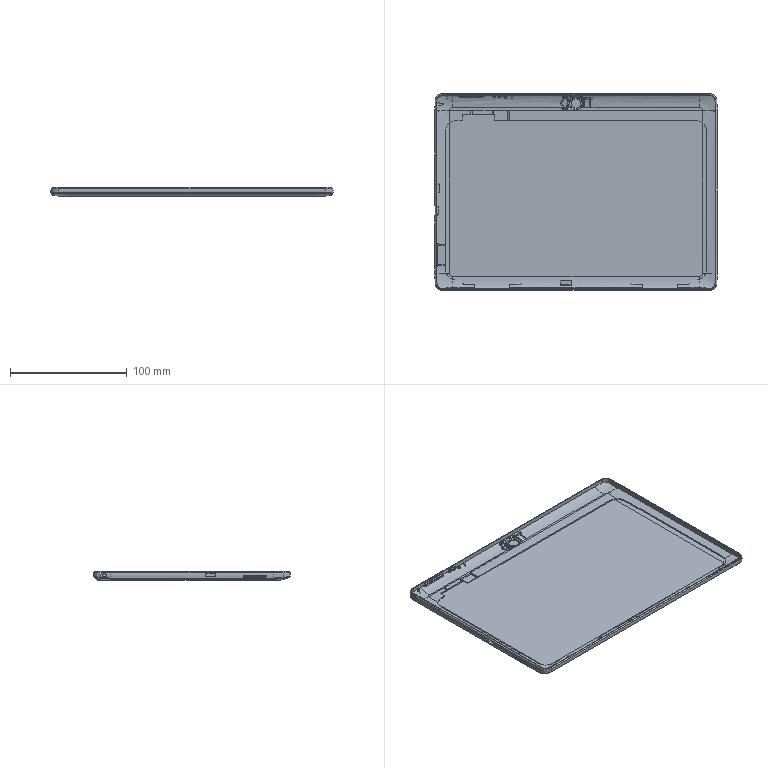Part | Creo | 1 solid | 439 faces | box 242.355 x 168.94 x 7.8 mm | volume 215366 mm3 | spline 166 | plane 161 | cylinder 66 | other 36 | cone 8 | torus 2 | commonest cylinder face diameters 2.2 x8 0.8 x6 0.6 x5 2.194 x4 2.6 x4 3.6 x4